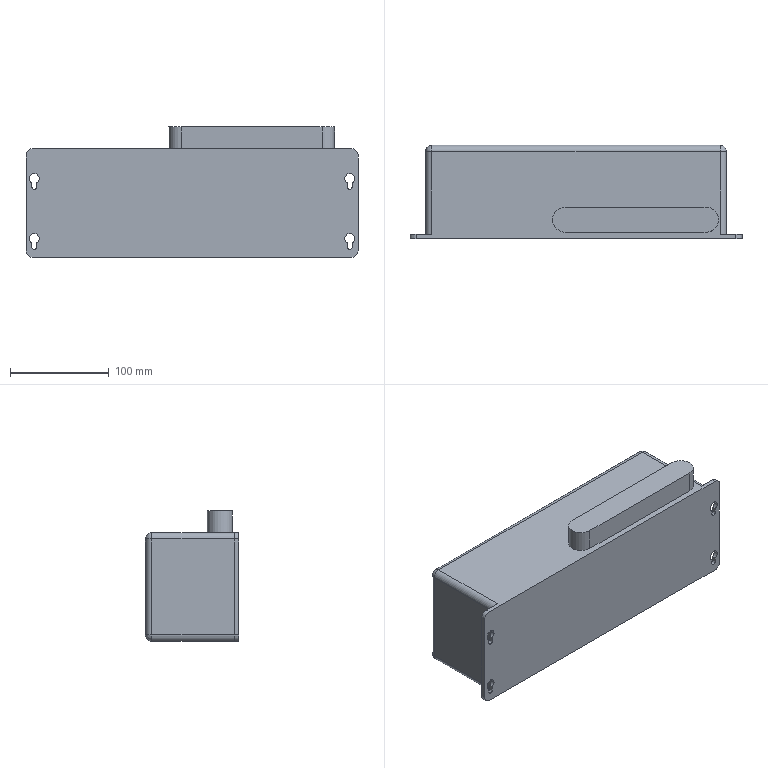Part | NX | features BREP 1 | 1 solid | 56 faces | box 336.55 x 94.488 x 132.207 mm | volume 3261574 mm3 | cylinder 31 | plane 21 | sphere 4 | commonest cylinder face diameters 9.982 x12 12.7 x12 4.978 x4 25.4 x3